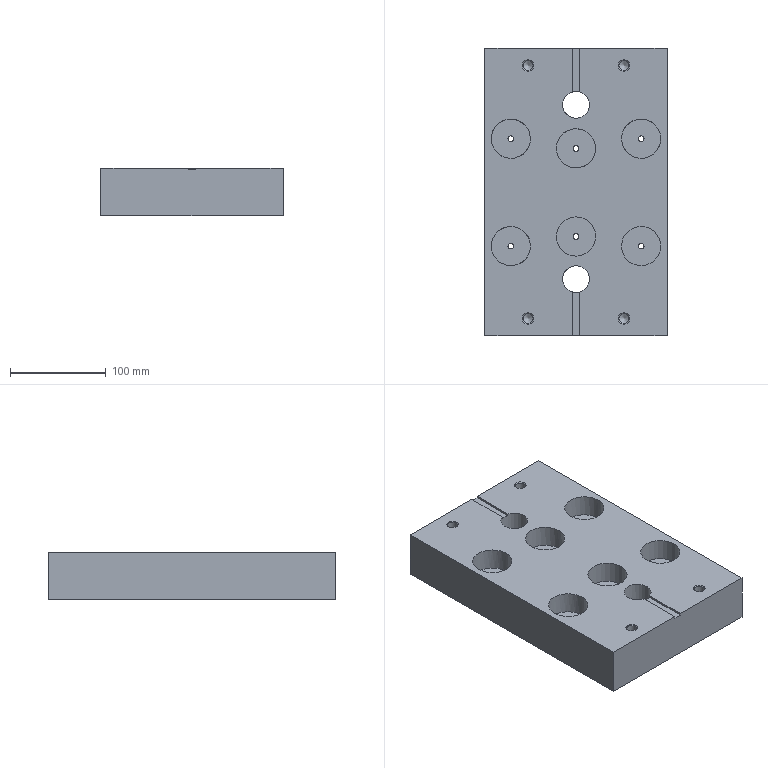Part | STEP file | gslz 2016.10.28-6_id1038_x_t | 1 solid | 44 faces | box 190 x 300 x 50 mm | volume 2589810 mm3 | plane 18 | cylinder 18 | cone 8 | commonest cylinder face diameters 6 x6 41 x6 10.3 x4 28 x2
STEP:
#1=CARTESIAN_POINT('',(4.,0.,-52.));
#2=VERTEX_POINT('',#1);
#3=CARTESIAN_POINT('',(-4.,0.,-52.));
#4=VERTEX_POINT('',#3);
#5=CARTESIAN_POINT('',(0.,0.,-52.));
#6=DIRECTION('',(-1.,0.,0.));
#7=VECTOR('',#6,1.);
#8=LINE('',#5,#7);
#9=EDGE_CURVE('',#2,#4,#8,.T.);
#10=ORIENTED_EDGE('',*,*,#9,.T.);
#11=CARTESIAN_POINT('',(-4.,0.,-50.));
#12=VERTEX_POINT('',#11);
#13=CARTESIAN_POINT('',(-4.,0.,-54.));
#14=DIRECTION('',(0.,0.,1.));
#15=VECTOR('',#14,1.);
#16=LINE('',#13,#15);
#17=EDGE_CURVE('',#4,#12,#16,.T.);
#18=ORIENTED_EDGE('',*,*,#17,.T.);
#19=CARTESIAN_POINT('',(-95.,0.,-50.));
#20=VERTEX_POINT('',#19);
#21=CARTESIAN_POINT('',(0.,0.,-50.));
#22=DIRECTION('',(1.,0.,0.));
#23=VECTOR('',#22,1.);
#24=LINE('',#21,#23);
#25=EDGE_CURVE('',#20,#12,#24,.T.);
#26=ORIENTED_EDGE('',*,*,#25,.F.);
#27=CARTESIAN_POINT('',(-95.,0.,-100.));
#28=VERTEX_POINT('',#27);
#29=CARTESIAN_POINT('',(-95.,0.,-221.492));
#30=DIRECTION('',(0.,0.,1.));
#31=VECTOR('',#30,1.);
#32=LINE('',#29,#31);
#33=EDGE_CURVE('',#28,#20,#32,.T.);
#34=ORIENTED_EDGE('',*,*,#33,.F.);
#35=CARTESIAN_POINT('',(95.,0.,-100.));
#36=VERTEX_POINT('',#35);
#37=CARTESIAN_POINT('',(0.,0.,-100.));
#38=DIRECTION('',(1.,0.,0.));
#39=VECTOR('',#38,1.);
#40=LINE('',#37,#39);
#41=EDGE_CURVE('',#28,#36,#40,.T.);
#42=ORIENTED_EDGE('',*,*,#41,.T.);
#43=CARTESIAN_POINT('',(95.,0.,-50.));
#44=VERTEX_POINT('',#43);
#45=CARTESIAN_POINT('',(95.,0.,-221.492));
#46=DIRECTION('',(0.,0.,1.));
#47=VECTOR('',#46,1.);
#48=LINE('',#45,#47);
#49=EDGE_CURVE('',#36,#44,#48,.T.);
#50=ORIENTED_EDGE('',*,*,#49,.T.);
#51=CARTESIAN_POINT('',(4.,0.,-50.));
#52=VERTEX_POINT('',#51);
#53=CARTESIAN_POINT('',(0.,0.,-50.));
#54=DIRECTION('',(1.,0.,0.));
#55=VECTOR('',#54,1.);
#56=LINE('',#53,#55);
#57=EDGE_CURVE('',#52,#44,#56,.T.);
#58=ORIENTED_EDGE('',*,*,#57,.F.);
#59=CARTESIAN_POINT('',(4.,0.,-54.));
#60=DIRECTION('',(0.,0.,1.));
#61=VECTOR('',#60,1.);
#62=LINE('',#59,#61);
#63=EDGE_CURVE('',#2,#52,#62,.T.);
#64=ORIENTED_EDGE('',*,*,#63,.F.);
#65=EDGE_LOOP('',(#10,#18,#26,#34,#42,#50,#58,#64));
#66=FACE_OUTER_BOUND('',#65,.T.);
#67=CARTESIAN_POINT('',(0.,0.,-221.492));
#68=DIRECTION('',(0.,-1.,0.));
#69=DIRECTION('',(0.,0.,1.));
#70=AXIS2_PLACEMENT_3D('',#67,#68,#69);
#71=PLANE('',#70);
#72=ADVANCED_FACE('',(#66),#71,.T.);
#73=CARTESIAN_POINT('',(-20.199,100.034,-50.));
#74=VERTEX_POINT('',#73);
#75=CARTESIAN_POINT('',(-0.000000001,103.534,-50.));
#76=DIRECTION('',(0.,0.,1.));
#77=DIRECTION('',(-1.,0.,0.));
#78=AXIS2_PLACEMENT_3D('',#75,#76,#77);
#79=CIRCLE('',#78,20.5);
#80=EDGE_CURVE('',#74,#74,#79,.T.);
#81=ORIENTED_EDGE('',*,*,#80,.F.);
#82=EDGE_LOOP('',(#81));
#83=FACE_BOUND('',#82,.T.);
#84=CARTESIAN_POINT('',(47.801,90.034,-50.));
#85=VERTEX_POINT('',#84);
#86=CARTESIAN_POINT('',(68.,93.534,-50.));
#87=DIRECTION('',(0.,0.,1.));
#88=DIRECTION('',(-1.,0.,0.));
#89=AXIS2_PLACEMENT_3D('',#86,#87,#88);
#90=CIRCLE('',#89,20.5);
#91=EDGE_CURVE('',#85,#85,#90,.T.);
#92=ORIENTED_EDGE('',*,*,#91,.F.);
#93=EDGE_LOOP('',(#92));
#94=FACE_BOUND('',#93,.T.);
#95=CARTESIAN_POINT('',(47.801,209.033,-50.));
#96=VERTEX_POINT('',#95);
#97=CARTESIAN_POINT('',(68.,205.533,-50.));
#98=DIRECTION('',(0.,0.,1.));
#99=DIRECTION('',(-1.,0.,0.));
#100=AXIS2_PLACEMENT_3D('',#97,#98,#99);
#101=CIRCLE('',#100,20.5);
#102=EDGE_CURVE('',#96,#96,#101,.T.);
#103=ORIENTED_EDGE('',*,*,#102,.F.);
#104=EDGE_LOOP('',(#103));
#105=FACE_BOUND('',#104,.T.);
#106=CARTESIAN_POINT('',(-20.199,199.033,-50.));
#107=VERTEX_POINT('',#106);
#108=CARTESIAN_POINT('',(0.,195.533,-50.));
#109=DIRECTION('',(0.,0.,-1.));
#110=DIRECTION('',(-1.,0.,0.));
#111=AXIS2_PLACEMENT_3D('',#108,#109,#110);
#112=CIRCLE('',#111,20.5);
#113=EDGE_CURVE('',#107,#107,#112,.T.);
#114=ORIENTED_EDGE('',*,*,#113,.T.);
#115=EDGE_LOOP('',(#114));
#116=FACE_BOUND('',#115,.T.);
#117=CARTESIAN_POINT('',(-47.801,90.034,-50.));
#118=VERTEX_POINT('',#117);
#119=CARTESIAN_POINT('',(-68.,93.534,-50.));
#120=DIRECTION('',(0.,0.,-1.));
#121=DIRECTION('',(-1.,0.,0.));
#122=AXIS2_PLACEMENT_3D('',#119,#120,#121);
#123=CIRCLE('',#122,20.5);
#124=EDGE_CURVE('',#118,#118,#123,.T.);
#125=ORIENTED_EDGE('',*,*,#124,.T.);
#126=EDGE_LOOP('',(#125));
#127=FACE_BOUND('',#126,.T.);
#128=CARTESIAN_POINT('',(4.,254.417,-50.));
#129=VERTEX_POINT('',#128);
#130=CARTESIAN_POINT('',(-4.,254.416,-50.));
#131=VERTEX_POINT('',#130);
#132=CARTESIAN_POINT('',(-0.000000005,241.,-50.));
#133=DIRECTION('',(0.,0.,-1.));
#134=DIRECTION('',(-1.,0.,0.));
#135=AXIS2_PLACEMENT_3D('',#132,#133,#134);
#136=CIRCLE('',#135,14.);
#137=EDGE_CURVE('',#129,#131,#136,.T.);
#138=ORIENTED_EDGE('',*,*,#137,.T.);
#139=CARTESIAN_POINT('',(-4.,300.,-50.));
#140=VERTEX_POINT('',#139);
#141=CARTESIAN_POINT('',(-4.,150.,-50.));
#142=DIRECTION('',(0.,-1.,0.));
#143=VECTOR('',#142,1.);
#144=LINE('',#141,#143);
#145=EDGE_CURVE('',#140,#131,#144,.T.);
#146=ORIENTED_EDGE('',*,*,#145,.F.);
#147=CARTESIAN_POINT('',(-95.,300.,-50.));
#148=VERTEX_POINT('',#147);
#149=CARTESIAN_POINT('',(0.,300.,-50.));
#150=DIRECTION('',(-1.,0.,0.));
#151=VECTOR('',#150,1.);
#152=LINE('',#149,#151);
#153=EDGE_CURVE('',#140,#148,#152,.T.);
#154=ORIENTED_EDGE('',*,*,#153,.T.);
#155=CARTESIAN_POINT('',(-95.,150.,-50.));
#156=DIRECTION('',(0.,1.,0.));
#157=VECTOR('',#156,1.);
#158=LINE('',#155,#157);
#159=EDGE_CURVE('',#20,#148,#158,.T.);
#160=ORIENTED_EDGE('',*,*,#159,.F.);
#161=ORIENTED_EDGE('',*,*,#25,.T.);
#162=CARTESIAN_POINT('',(-4.,45.584,-50.));
#163=VERTEX_POINT('',#162);
#164=CARTESIAN_POINT('',(-4.,150.,-50.));
#165=DIRECTION('',(0.,1.,0.));
#166=VECTOR('',#165,1.);
#167=LINE('',#164,#166);
#168=EDGE_CURVE('',#12,#163,#167,.T.);
#169=ORIENTED_EDGE('',*,*,#168,.T.);
#170=CARTESIAN_POINT('',(4.,45.583,-50.));
#171=VERTEX_POINT('',#170);
#172=CARTESIAN_POINT('',(0.000000001,59.,-50.));
#173=DIRECTION('',(0.,0.,-1.));
#174=DIRECTION('',(-1.,0.,0.));
#175=AXIS2_PLACEMENT_3D('',#172,#173,#174);
#176=CIRCLE('',#175,14.);
#177=EDGE_CURVE('',#163,#171,#176,.T.);
#178=ORIENTED_EDGE('',*,*,#177,.T.);
#179=CARTESIAN_POINT('',(4.,150.,-50.));
#180=DIRECTION('',(0.,1.,0.));
#181=VECTOR('',#180,1.);
#182=LINE('',#179,#181);
#183=EDGE_CURVE('',#52,#171,#182,.T.);
#184=ORIENTED_EDGE('',*,*,#183,.F.);
#185=ORIENTED_EDGE('',*,*,#57,.T.);
#186=CARTESIAN_POINT('',(95.,300.,-50.));
#187=VERTEX_POINT('',#186);
#188=CARTESIAN_POINT('',(95.,150.,-50.));
#189=DIRECTION('',(0.,1.,0.));
#190=VECTOR('',#189,1.);
#191=LINE('',#188,#190);
#192=EDGE_CURVE('',#44,#187,#191,.T.);
#193=ORIENTED_EDGE('',*,*,#192,.T.);
#194=CARTESIAN_POINT('',(4.,300.,-50.));
#195=VERTEX_POINT('',#194);
#196=CARTESIAN_POINT('',(0.,300.,-50.));
#197=DIRECTION('',(-1.,0.,0.));
#198=VECTOR('',#197,1.);
#199=LINE('',#196,#198);
#200=EDGE_CURVE('',#187,#195,#199,.T.);
#201=ORIENTED_EDGE('',*,*,#200,.T.);
#202=CARTESIAN_POINT('',(4.,150.,-50.));
#203=DIRECTION('',(0.,-1.,0.));
#204=VECTOR('',#203,1.);
#205=LINE('',#202,#204);
#206=EDGE_CURVE('',#195,#129,#205,.T.);
#207=ORIENTED_EDGE('',*,*,#206,.T.);
#208=EDGE_LOOP('',(#138,#146,#154,#160,#161,#169,#178,#184,#185,#193,#201,#207));
#209=FACE_BOUND('',#208,.T.);
#210=CARTESIAN_POINT('',(-47.801,202.033,-50.));
#211=VERTEX_POINT('',#210);
#212=CARTESIAN_POINT('',(-68.,205.533,-50.));
#213=DIRECTION('',(0.,0.,-1.));
#214=DIRECTION('',(-1.,0.,0.));
#215=AXIS2_PLACEMENT_3D('',#212,#213,#214);
#216=CIRCLE('',#215,20.5);
#217=EDGE_CURVE('',#211,#211,#216,.T.);
#218=ORIENTED_EDGE('',*,*,#217,.T.);
#219=EDGE_LOOP('',(#218));
#220=FACE_BOUND('',#219,.T.);
#221=CARTESIAN_POINT('',(44.,282.,-50.));
#222=VERTEX_POINT('',#221);
#223=CARTESIAN_POINT('',(50.,282.,-50.));
#224=DIRECTION('',(0.,0.,1.));
#225=DIRECTION('',(-1.,0.,0.));
#226=AXIS2_PLACEMENT_3D('',#223,#224,#225);
#227=CIRCLE('',#226,6.);
#228=EDGE_CURVE('',#222,#222,#227,.T.);
#229=ORIENTED_EDGE('',*,*,#228,.F.);
#230=EDGE_LOOP('',(#229));
#231=FACE_BOUND('',#230,.T.);
#232=CARTESIAN_POINT('',(-56.,282.,-50.));
#233=VERTEX_POINT('',#232);
#234=CARTESIAN_POINT('',(-50.,282.,-50.));
#235=DIRECTION('',(0.,0.,1.));
#236=DIRECTION('',(-1.,0.,0.));
#237=AXIS2_PLACEMENT_3D('',#234,#235,#236);
#238=CIRCLE('',#237,6.);
#239=EDGE_CURVE('',#233,#233,#238,.T.);
#240=ORIENTED_EDGE('',*,*,#239,.F.);
#241=EDGE_LOOP('',(#240));
#242=FACE_BOUND('',#241,.T.);
#243=CARTESIAN_POINT('',(44.,18.,-50.));
#244=VERTEX_POINT('',#243);
#245=CARTESIAN_POINT('',(50.,18.,-50.));
#246=DIRECTION('',(0.,0.,1.));
#247=DIRECTION('',(-1.,0.,0.));
#248=AXIS2_PLACEMENT_3D('',#245,#246,#247);
#249=CIRCLE('',#248,6.);
#250=EDGE_CURVE('',#244,#244,#249,.T.);
#251=ORIENTED_EDGE('',*,*,#250,.F.);
#252=EDGE_LOOP('',(#251));
#253=FACE_BOUND('',#252,.T.);
#254=CARTESIAN_POINT('',(-56.,18.,-50.));
#255=VERTEX_POINT('',#254);
#256=CARTESIAN_POINT('',(-50.,18.,-50.));
#257=DIRECTION('',(0.,0.,1.));
#258=DIRECTION('',(-1.,0.,0.));
#259=AXIS2_PLACEMENT_3D('',#256,#257,#258);
#260=CIRCLE('',#259,6.);
#261=EDGE_CURVE('',#255,#255,#260,.T.);
#262=ORIENTED_EDGE('',*,*,#261,.F.);
#263=EDGE_LOOP('',(#262));
#264=FACE_BOUND('',#263,.T.);
#265=CARTESIAN_POINT('',(-10.,150.,-50.));
#266=DIRECTION('',(0.,0.,-1.));
#267=DIRECTION('',(1.,0.,0.));
#268=AXIS2_PLACEMENT_3D('',#265,#266,#267);
#269=PLANE('',#268);
#270=ADVANCED_FACE('',(#83,#94,#105,#116,#127,#209,#220,#231,#242,#253,#264),#269,.F.);
#271=CARTESIAN_POINT('',(-4.,300.,-52.));
#272=VERTEX_POINT('',#271);
#273=CARTESIAN_POINT('',(4.,300.,-52.));
#274=VERTEX_POINT('',#273);
#275=CARTESIAN_POINT('',(0.,300.,-52.));
#276=DIRECTION('',(1.,0.,0.));
#277=VECTOR('',#276,1.);
#278=LINE('',#275,#277);
#279=EDGE_CURVE('',#272,#274,#278,.T.);
#280=ORIENTED_EDGE('',*,*,#279,.T.);
#281=CARTESIAN_POINT('',(4.,300.,-54.));
#282=DIRECTION('',(0.,0.,1.));
#283=VECTOR('',#282,1.);
#284=LINE('',#281,#283);
#285=EDGE_CURVE('',#274,#195,#284,.T.);
#286=ORIENTED_EDGE('',*,*,#285,.T.);
#287=ORIENTED_EDGE('',*,*,#200,.F.);
#288=CARTESIAN_POINT('',(95.,300.,-100.));
#289=VERTEX_POINT('',#288);
#290=CARTESIAN_POINT('',(95.,300.,-221.492));
#291=DIRECTION('',(0.,0.,1.));
#292=VECTOR('',#291,1.);
#293=LINE('',#290,#292);
#294=EDGE_CURVE('',#289,#187,#293,.T.);
#295=ORIENTED_EDGE('',*,*,#294,.F.);
#296=CARTESIAN_POINT('',(-95.,300.,-100.));
#297=VERTEX_POINT('',#296);
#298=CARTESIAN_POINT('',(0.,300.,-100.));
#299=DIRECTION('',(-1.,0.,0.));
#300=VECTOR('',#299,1.);
#301=LINE('',#298,#300);
#302=EDGE_CURVE('',#289,#297,#301,.T.);
#303=ORIENTED_EDGE('',*,*,#302,.T.);
#304=CARTESIAN_POINT('',(-95.,300.,-221.492));
#305=DIRECTION('',(0.,0.,1.));
#306=VECTOR('',#305,1.);
#307=LINE('',#304,#306);
#308=EDGE_CURVE('',#297,#148,#307,.T.);
#309=ORIENTED_EDGE('',*,*,#308,.T.);
#310=ORIENTED_EDGE('',*,*,#153,.F.);
#311=CARTESIAN_POINT('',(-4.,300.,-54.));
#312=DIRECTION('',(0.,0.,1.));
#313=VECTOR('',#312,1.);
#314=LINE('',#311,#313);
#315=EDGE_CURVE('',#272,#140,#314,.T.);
#316=ORIENTED_EDGE('',*,*,#315,.F.);
#317=EDGE_LOOP('',(#280,#286,#287,#295,#303,#309,#310,#316));
#318=FACE_OUTER_BOUND('',#317,.T.);
#319=CARTESIAN_POINT('',(0.,300.,-221.492));
#320=DIRECTION('',(0.,1.,0.));
#321=DIRECTION('',(0.,0.,-1.));
#322=AXIS2_PLACEMENT_3D('',#319,#320,#321);
#323=PLANE('',#322);
#324=ADVANCED_FACE('',(#318),#323,.T.);
#325=CARTESIAN_POINT('',(3.,103.534,-73.));
#326=VERTEX_POINT('',#325);
#327=CARTESIAN_POINT('',(-0.000000001,103.534,-73.));
#328=DIRECTION('',(0.,0.,1.));
#329=DIRECTION('',(1.,0.,0.));
#330=AXIS2_PLACEMENT_3D('',#327,#328,#329);
#331=CIRCLE('',#330,3.);
#332=EDGE_CURVE('',#326,#326,#331,.T.);
#333=ORIENTED_EDGE('',*,*,#332,.F.);
#334=EDGE_LOOP('',(#333));
#335=FACE_BOUND('',#334,.T.);
#336=CARTESIAN_POINT('',(-20.201,100.046,-73.));
#337=VERTEX_POINT('',#336);
#338=CARTESIAN_POINT('',(-20.199,100.034,-73.));
#339=VERTEX_POINT('',#338);
#340=CARTESIAN_POINT('',(-0.000000001,103.534,-73.));
#341=DIRECTION('',(0.,0.,-1.));
#342=DIRECTION('',(1.,0.,0.));
#343=AXIS2_PLACEMENT_3D('',#340,#341,#342);
#344=CIRCLE('',#343,20.5);
#345=EDGE_CURVE('',#337,#339,#344,.T.);
#346=ORIENTED_EDGE('',*,*,#345,.F.);
#347=CARTESIAN_POINT('',(-0.000000001,103.534,-73.));
#348=DIRECTION('',(0.,0.,-1.));
#349=DIRECTION('',(1.,0.,0.));
#350=AXIS2_PLACEMENT_3D('',#347,#348,#349);
#351=CIRCLE('',#350,20.5);
#352=EDGE_CURVE('',#339,#337,#351,.T.);
#353=ORIENTED_EDGE('',*,*,#352,.F.);
#354=EDGE_LOOP('',(#346,#353));
#355=FACE_BOUND('',#354,.T.);
#356=CARTESIAN_POINT('',(-0.000000001,103.534,-73.));
#357=DIRECTION('',(0.,0.,1.));
#358=DIRECTION('',(-1.,0.,0.));
#359=AXIS2_PLACEMENT_3D('',#356,#357,#358);
#360=PLANE('',#359);
#361=ADVANCED_FACE('',(#335,#355),#360,.T.);
#362=CARTESIAN_POINT('',(-65.,205.533,-73.));
#363=VERTEX_POINT('',#362);
#364=CARTESIAN_POINT('',(-68.,205.533,-73.));
#365=DIRECTION('',(0.,0.,1.));
#366=DIRECTION('',(1.,0.,0.));
#367=AXIS2_PLACEMENT_3D('',#364,#365,#366);
#368=CIRCLE('',#367,3.);
#369=EDGE_CURVE('',#363,#363,#368,.T.);
#370=ORIENTED_EDGE('',*,*,#369,.F.);
#371=EDGE_LOOP('',(#370));
#372=FACE_BOUND('',#371,.T.);
#373=CARTESIAN_POINT('',(-47.799,209.02,-73.));
#374=VERTEX_POINT('',#373);
#375=CARTESIAN_POINT('',(-47.801,202.033,-73.));
#376=VERTEX_POINT('',#375);
#377=CARTESIAN_POINT('',(-68.,205.533,-73.));
#378=DIRECTION('',(0.,0.,-1.));
#379=DIRECTION('',(1.,0.,0.));
#380=AXIS2_PLACEMENT_3D('',#377,#378,#379);
#381=CIRCLE('',#380,20.5);
#382=EDGE_CURVE('',#374,#376,#381,.T.);
#383=ORIENTED_EDGE('',*,*,#382,.F.);
#384=CARTESIAN_POINT('',(-68.,205.533,-73.));
#385=DIRECTION('',(0.,0.,-1.));
#386=DIRECTION('',(1.,0.,0.));
#387=AXIS2_PLACEMENT_3D('',#384,#385,#386);
#388=CIRCLE('',#387,20.5);
#389=EDGE_CURVE('',#376,#374,#388,.T.);
#390=ORIENTED_EDGE('',*,*,#389,.F.);
#391=EDGE_LOOP('',(#383,#390));
#392=FACE_BOUND('',#391,.T.);
#393=CARTESIAN_POINT('',(-107.5,104.533,-73.));
#394=DIRECTION('',(0.,0.,1.));
#395=DIRECTION('',(-1.,0.,0.));
#396=AXIS2_PLACEMENT_3D('',#393,#394,#395);
#397=PLANE('',#396);
#398=ADVANCED_FACE('',(#372,#392),#397,.T.);
#399=CARTESIAN_POINT('',(-65.,93.534,-73.));
#400=VERTEX_POINT('',#399);
#401=CARTESIAN_POINT('',(-68.,93.534,-73.));
#402=DIRECTION('',(0.,0.,1.));
#403=DIRECTION('',(1.,0.,0.));
#404=AXIS2_PLACEMENT_3D('',#401,#402,#403);
#405=CIRCLE('',#404,3.);
#406=EDGE_CURVE('',#400,#400,#405,.T.);
#407=ORIENTED_EDGE('',*,*,#406,.F.);
#408=EDGE_LOOP('',(#407));
#409=FACE_BOUND('',#408,.T.);
#410=CARTESIAN_POINT('',(-47.799,97.021,-73.));
#411=VERTEX_POINT('',#410);
#412=CARTESIAN_POINT('',(-47.801,90.034,-73.));
#413=VERTEX_POINT('',#412);
#414=CARTESIAN_POINT('',(-68.,93.534,-73.));
#415=DIRECTION('',(0.,0.,-1.));
#416=DIRECTION('',(1.,0.,0.));
#417=AXIS2_PLACEMENT_3D('',#414,#415,#416);
#418=CIRCLE('',#417,20.5);
#419=EDGE_CURVE('',#411,#413,#418,.T.);
#420=ORIENTED_EDGE('',*,*,#419,.F.);
#421=CARTESIAN_POINT('',(-68.,93.534,-73.));
#422=DIRECTION('',(0.,0.,-1.));
#423=DIRECTION('',(1.,0.,0.));
#424=AXIS2_PLACEMENT_3D('',#421,#422,#423);
#425=CIRCLE('',#424,20.5);
#426=EDGE_CURVE('',#413,#411,#425,.T.);
#427=ORIENTED_EDGE('',*,*,#426,.F.);
#428=EDGE_LOOP('',(#420,#427));
#429=FACE_BOUND('',#428,.T.);
#430=CARTESIAN_POINT('',(-107.5,96.534,-73.));
#431=DIRECTION('',(0.,0.,1.));
#432=DIRECTION('',(-1.,0.,0.));
#433=AXIS2_PLACEMENT_3D('',#430,#431,#432);
#434=PLANE('',#433);
#435=ADVANCED_FACE('',(#409,#429),#434,.T.);
#436=CARTESIAN_POINT('',(71.,93.534,-73.));
#437=VERTEX_POINT('',#436);
#438=CARTESIAN_POINT('',(68.,93.534,-73.));
#439=DIRECTION('',(0.,0.,1.));
#440=DIRECTION('',(1.,0.,0.));
#441=AXIS2_PLACEMENT_3D('',#438,#439,#440);
#442=CIRCLE('',#441,3.);
#443=EDGE_CURVE('',#437,#437,#442,.T.);
#444=ORIENTED_EDGE('',*,*,#443,.F.);
#445=EDGE_LOOP('',(#444));
#446=FACE_BOUND('',#445,.T.);
#447=CARTESIAN_POINT('',(47.799,90.046,-73.));
#448=VERTEX_POINT('',#447);
#449=CARTESIAN_POINT('',(47.801,90.034,-73.));
#450=VERTEX_POINT('',#449);
#451=CARTESIAN_POINT('',(68.,93.534,-73.));
#452=DIRECTION('',(0.,0.,-1.));
#453=DIRECTION('',(1.,0.,0.));
#454=AXIS2_PLACEMENT_3D('',#451,#452,#453);
#455=CIRCLE('',#454,20.5);
#456=EDGE_CURVE('',#448,#450,#455,.T.);
#457=ORIENTED_EDGE('',*,*,#456,.F.);
#458=CARTESIAN_POINT('',(68.,93.534,-73.));
#459=DIRECTION('',(0.,0.,-1.));
#460=DIRECTION('',(1.,0.,0.));
#461=AXIS2_PLACEMENT_3D('',#458,#459,#460);
#462=CIRCLE('',#461,20.5);
#463=EDGE_CURVE('',#450,#448,#462,.T.);
#464=ORIENTED_EDGE('',*,*,#463,.F.);
#465=EDGE_LOOP('',(#457,#464));
#466=FACE_BOUND('',#465,.T.);
#467=CARTESIAN_POINT('',(68.,93.534,-73.));
#468=DIRECTION('',(0.,0.,1.));
#469=DIRECTION('',(-1.,0.,0.));
#470=AXIS2_PLACEMENT_3D('',#467,#468,#469);
#471=PLANE('',#470);
#472=ADVANCED_FACE('',(#446,#466),#471,.T.);
#473=CARTESIAN_POINT('',(71.,205.533,-73.));
#474=VERTEX_POINT('',#473);
#475=CARTESIAN_POINT('',(68.,205.533,-73.));
#476=DIRECTION('',(0.,0.,1.));
#477=DIRECTION('',(1.,0.,0.));
#478=AXIS2_PLACEMENT_3D('',#475,#476,#477);
#479=CIRCLE('',#478,3.);
#480=EDGE_CURVE('',#474,#474,#479,.T.);
#481=ORIENTED_EDGE('',*,*,#480,.F.);
#482=EDGE_LOOP('',(#481));
#483=FACE_BOUND('',#482,.T.);
#484=CARTESIAN_POINT('',(47.799,202.046,-73.));
#485=VERTEX_POINT('',#484);
#486=CARTESIAN_POINT('',(47.801,209.033,-73.));
#487=VERTEX_POINT('',#486);
#488=CARTESIAN_POINT('',(68.,205.533,-73.));
#489=DIRECTION('',(0.,0.,-1.));
#490=DIRECTION('',(1.,0.,0.));
#491=AXIS2_PLACEMENT_3D('',#488,#489,#490);
#492=CIRCLE('',#491,20.5);
#493=EDGE_CURVE('',#485,#487,#492,.T.);
#494=ORIENTED_EDGE('',*,*,#493,.F.);
#495=CARTESIAN_POINT('',(68.,205.533,-73.));
#496=DIRECTION('',(0.,0.,-1.));
#497=DIRECTION('',(1.,0.,0.));
#498=AXIS2_PLACEMENT_3D('',#495,#496,#497);
#499=CIRCLE('',#498,20.5);
#500=EDGE_CURVE('',#487,#485,#499,.T.);
#501=ORIENTED_EDGE('',*,*,#500,.F.);
#502=EDGE_LOOP('',(#494,#501));
#503=FACE_BOUND('',#502,.T.);
#504=CARTESIAN_POINT('',(68.,205.533,-73.));
#505=DIRECTION('',(0.,0.,1.));
#506=DIRECTION('',(-1.,0.,0.));
#507=AXIS2_PLACEMENT_3D('',#504,#505,#506);
#508=PLANE('',#507);
#509=ADVANCED_FACE('',(#483,#503),#508,.T.);
#510=CARTESIAN_POINT('',(-3.,195.533,-73.));
#511=VERTEX_POINT('',#510);
#512=CARTESIAN_POINT('',(0.,195.533,-73.));
#513=DIRECTION('',(0.,0.,-1.));
#514=DIRECTION('',(-1.,0.,0.));
#515=AXIS2_PLACEMENT_3D('',#512,#513,#514);
#516=CIRCLE('',#515,3.);
#517=EDGE_CURVE('',#511,#511,#516,.T.);
#518=ORIENTED_EDGE('',*,*,#517,.T.);
#519=EDGE_LOOP('',(#518));
#520=FACE_BOUND('',#519,.T.);
#521=CARTESIAN_POINT('',(-20.199,199.033,-73.));
#522=VERTEX_POINT('',#521);
#523=CARTESIAN_POINT('',(-20.201,192.046,-73.));
#524=VERTEX_POINT('',#523);
#525=CARTESIAN_POINT('',(0.,195.533,-73.));
#526=DIRECTION('',(0.,0.,1.));
#527=DIRECTION('',(-1.,0.,0.));
#528=AXIS2_PLACEMENT_3D('',#525,#526,#527);
#529=CIRCLE('',#528,20.5);
#530=EDGE_CURVE('',#522,#524,#529,.T.);
#531=ORIENTED_EDGE('',*,*,#530,.T.);
#532=CARTESIAN_POINT('',(0.,195.533,-73.));
#533=DIRECTION('',(0.,0.,1.));
#534=DIRECTION('',(-1.,0.,0.));
#535=AXIS2_PLACEMENT_3D('',#532,#533,#534);
#536=CIRCLE('',#535,20.5);
#537=EDGE_CURVE('',#524,#522,#536,.T.);
#538=ORIENTED_EDGE('',*,*,#537,.T.);
#539=EDGE_LOOP('',(#531,#538));
#540=FACE_BOUND('',#539,.T.);
#541=CARTESIAN_POINT('',(0.,195.533,-73.));
#542=DIRECTION('',(0.,0.,-1.));
#543=DIRECTION('',(1.,0.,0.));
#544=AXIS2_PLACEMENT_3D('',#541,#542,#543);
#545=PLANE('',#544);
#546=ADVANCED_FACE('',(#520,#540),#545,.F.);
#547=CARTESIAN_POINT('',(-71.,93.534,-100.));
#548=VERTEX_POINT('',#547);
#549=CARTESIAN_POINT('',(-68.,93.534,-100.));
#550=DIRECTION('',(0.,0.,-1.));
#551=DIRECTION('',(-1.,0.,0.));
#552=AXIS2_PLACEMENT_3D('',#549,#550,#551);
#553=CIRCLE('',#552,3.);
#554=EDGE_CURVE('',#548,#548,#553,.T.);
#555=ORIENTED_EDGE('',*,*,#554,.F.);
#556=EDGE_LOOP('',(#555));
#557=FACE_BOUND('',#556,.T.);
#558=CARTESIAN_POINT('',(-71.,205.533,-100.));
#559=VERTEX_POINT('',#558);
#560=CARTESIAN_POINT('',(-68.,205.533,-100.));
#561=DIRECTION('',(0.,0.,-1.));
#562=DIRECTION('',(-1.,0.,0.));
#563=AXIS2_PLACEMENT_3D('',#560,#561,#562);
#564=CIRCLE('',#563,3.);
#565=EDGE_CURVE('',#559,#559,#564,.T.);
#566=ORIENTED_EDGE('',*,*,#565,.F.);
#567=EDGE_LOOP('',(#566));
#568=FACE_BOUND('',#567,.T.);
#569=CARTESIAN_POINT('',(65.,205.533,-100.));
#570=VERTEX_POINT('',#569);
#571=CARTESIAN_POINT('',(68.,205.533,-100.));
#572=DIRECTION('',(0.,0.,-1.));
#573=DIRECTION('',(-1.,0.,0.));
#574=AXIS2_PLACEMENT_3D('',#571,#572,#573);
#575=CIRCLE('',#574,3.);
#576=EDGE_CURVE('',#570,#570,#575,.T.);
#577=ORIENTED_EDGE('',*,*,#576,.F.);
#578=EDGE_LOOP('',(#577));
#579=FACE_BOUND('',#578,.T.);
#580=CARTESIAN_POINT('',(-3.,195.533,-100.));
#581=VERTEX_POINT('',#580);
#582=CARTESIAN_POINT('',(0.,195.533,-100.));
#583=DIRECTION('',(0.,0.,-1.));
#584=DIRECTION('',(-1.,0.,0.));
#585=AXIS2_PLACEMENT_3D('',#582,#583,#584);
#586=CIRCLE('',#585,3.);
#587=EDGE_CURVE('',#581,#581,#586,.T.);
#588=ORIENTED_EDGE('',*,*,#587,.F.);
#589=EDGE_LOOP('',(#588));
#590=FACE_BOUND('',#589,.T.);
#591=CARTESIAN_POINT('',(-3.,103.534,-100.));
#592=VERTEX_POINT('',#591);
#593=CARTESIAN_POINT('',(-0.000000001,103.534,-100.));
#594=DIRECTION('',(0.,0.,-1.));
#595=DIRECTION('',(-1.,0.,0.));
#596=AXIS2_PLACEMENT_3D('',#593,#594,#595);
#597=CIRCLE('',#596,3.);
#598=EDGE_CURVE('',#592,#592,#597,.T.);
#599=ORIENTED_EDGE('',*,*,#598,.F.);
#600=EDGE_LOOP('',(#599));
#601=FACE_BOUND('',#600,.T.);
#602=CARTESIAN_POINT('',(65.,93.534,-100.));
#603=VERTEX_POINT('',#602);
#604=CARTESIAN_POINT('',(68.,93.534,-100.));
#605=DIRECTION('',(0.,0.,-1.));
#606=DIRECTION('',(-1.,0.,0.));
#607=AXIS2_PLACEMENT_3D('',#604,#605,#606);
#608=CIRCLE('',#607,3.);
#609=EDGE_CURVE('',#603,#603,#608,.T.);
#610=ORIENTED_EDGE('',*,*,#609,.F.);
#611=EDGE_LOOP('',(#610));
#612=FACE_BOUND('',#611,.T.);
#613=CARTESIAN_POINT('',(-14.,241.,-100.));
#614=VERTEX_POINT('',#613);
#615=CARTESIAN_POINT('',(-0.000000005,241.,-100.));
#616=DIRECTION('',(0.,0.,-1.));
#617=DIRECTION('',(-1.,0.,0.));
#618=AXIS2_PLACEMENT_3D('',#615,#616,#617);
#619=CIRCLE('',#618,14.);
#620=EDGE_CURVE('',#614,#614,#619,.T.);
#621=ORIENTED_EDGE('',*,*,#620,.F.);
#622=EDGE_LOOP('',(#621));
#623=FACE_BOUND('',#622,.T.);
#624=CARTESIAN_POINT('',(-14.,59.,-100.));
#625=VERTEX_POINT('',#624);
#626=CARTESIAN_POINT('',(0.000000001,59.,-100.));
#627=DIRECTION('',(0.,0.,-1.));
#628=DIRECTION('',(-1.,0.,0.));
#629=AXIS2_PLACEMENT_3D('',#626,#627,#628);
#630=CIRCLE('',#629,14.);
#631=EDGE_CURVE('',#625,#625,#630,.T.);
#632=ORIENTED_EDGE('',*,*,#631,.F.);
#633=EDGE_LOOP('',(#632));
#634=FACE_BOUND('',#633,.T.);
#635=CARTESIAN_POINT('',(-95.,150.,-100.));
#636=DIRECTION('',(0.,1.,0.));
#637=VECTOR('',#636,1.);
#638=LINE('',#635,#637);
#639=EDGE_CURVE('',#28,#297,#638,.T.);
#640=ORIENTED_EDGE('',*,*,#639,.T.);
#641=ORIENTED_EDGE('',*,*,#302,.F.);
#642=CARTESIAN_POINT('',(95.,150.,-100.));
#643=DIRECTION('',(0.,1.,0.));
#644=VECTOR('',#643,1.);
#645=LINE('',#642,#644);
#646=EDGE_CURVE('',#36,#289,#645,.T.);
#647=ORIENTED_EDGE('',*,*,#646,.F.);
#648=ORIENTED_EDGE('',*,*,#41,.F.);
#649=EDGE_LOOP('',(#640,#641,#647,#648));
#650=FACE_BOUND('',#649,.T.);
#651=CARTESIAN_POINT('',(-140.,150.,-100.));
#652=DIRECTION('',(0.,0.,-1.));
#653=DIRECTION('',(1.,0.,0.));
#654=AXIS2_PLACEMENT_3D('',#651,#652,#653);
#655=PLANE('',#654);
#656=ADVANCED_FACE('',(#557,#568,#579,#590,#601,#612,#623,#634,#650),#655,.T.);
#657=ORIENTED_EDGE('',*,*,#426,.T.);
#658=ORIENTED_EDGE('',*,*,#419,.T.);
#659=EDGE_LOOP('',(#657,#658));
#660=FACE_BOUND('',#659,.T.);
#661=ORIENTED_EDGE('',*,*,#124,.F.);
#662=EDGE_LOOP('',(#661));
#663=FACE_BOUND('',#662,.T.);
#664=CARTESIAN_POINT('',(-68.,93.534,278.));
#665=DIRECTION('',(0.,0.,1.));
#666=DIRECTION('',(1.,0.,0.));
#667=AXIS2_PLACEMENT_3D('',#664,#665,#666);
#668=CYLINDRICAL_SURFACE('',#667,20.5);
#669=ADVANCED_FACE('',(#660,#663),#668,.F.);
#670=ORIENTED_EDGE('',*,*,#389,.T.);
#671=ORIENTED_EDGE('',*,*,#382,.T.);
#672=EDGE_LOOP('',(#670,#671));
#673=FACE_BOUND('',#672,.T.);
#674=ORIENTED_EDGE('',*,*,#217,.F.);
#675=EDGE_LOOP('',(#674));
#676=FACE_BOUND('',#675,.T.);
#677=CARTESIAN_POINT('',(-68.,205.533,-27.));
#678=DIRECTION('',(0.,0.,1.));
#679=DIRECTION('',(-1.,0.,0.));
#680=AXIS2_PLACEMENT_3D('',#677,#678,#679);
#681=CYLINDRICAL_SURFACE('',#680,20.5);
#682=ADVANCED_FACE('',(#673,#676),#681,.F.);
#683=ORIENTED_EDGE('',*,*,#352,.T.);
#684=ORIENTED_EDGE('',*,*,#345,.T.);
#685=EDGE_LOOP('',(#683,#684));
#686=FACE_BOUND('',#685,.T.);
#687=ORIENTED_EDGE('',*,*,#80,.T.);
#688=EDGE_LOOP('',(#687));
#689=FACE_BOUND('',#688,.T.);
#690=CARTESIAN_POINT('',(-0.000000001,103.534,-73.));
#691=DIRECTION('',(0.,0.,1.));
#692=DIRECTION('',(-1.,0.,0.));
#693=AXIS2_PLACEMENT_3D('',#690,#691,#692);
#694=CYLINDRICAL_SURFACE('',#693,20.5);
#695=ADVANCED_FACE('',(#686,#689),#694,.F.);
#696=ORIENTED_EDGE('',*,*,#537,.F.);
#697=ORIENTED_EDGE('',*,*,#530,.F.);
#698=EDGE_LOOP('',(#696,#697));
#699=FACE_BOUND('',#698,.T.);
#700=ORIENTED_EDGE('',*,*,#113,.F.);
#701=EDGE_LOOP('',(#700));
#702=FACE_BOUND('',#701,.T.);
#703=CARTESIAN_POINT('',(0.,195.533,-73.));
#704=DIRECTION('',(0.,0.,1.));
#705=DIRECTION('',(-1.,0.,0.));
#706=AXIS2_PLACEMENT_3D('',#703,#704,#705);
#707=CYLINDRICAL_SURFACE('',#706,20.5);
#708=ADVANCED_FACE('',(#699,#702),#707,.F.);
#709=ORIENTED_EDGE('',*,*,#500,.T.);
#710=ORIENTED_EDGE('',*,*,#493,.T.);
#711=EDGE_LOOP('',(#709,#710));
#712=FACE_BOUND('',#711,.T.);
#713=ORIENTED_EDGE('',*,*,#102,.T.);
#714=EDGE_LOOP('',(#713));
#715=FACE_BOUND('',#714,.T.);
#716=CARTESIAN_POINT('',(68.,205.533,-73.));
#717=DIRECTION('',(0.,0.,1.));
#718=DIRECTION('',(-1.,0.,0.));
#719=AXIS2_PLACEMENT_3D('',#716,#717,#718);
#720=CYLINDRICAL_SURFACE('',#719,20.5);
#721=ADVANCED_FACE('',(#712,#715),#720,.F.);
#722=ORIENTED_EDGE('',*,*,#463,.T.);
#723=ORIENTED_EDGE('',*,*,#456,.T.);
#724=EDGE_LOOP('',(#722,#723));
#725=FACE_BOUND('',#724,.T.);
#726=ORIENTED_EDGE('',*,*,#91,.T.);
#727=EDGE_LOOP('',(#726));
#728=FACE_BOUND('',#727,.T.);
#729=CARTESIAN_POINT('',(68.,93.534,-73.));
#730=DIRECTION('',(0.,0.,1.));
#731=DIRECTION('',(-1.,0.,0.));
#732=AXIS2_PLACEMENT_3D('',#729,#730,#731);
#733=CYLINDRICAL_SURFACE('',#732,20.5);
#734=ADVANCED_FACE('',(#725,#728),#733,.F.);
#735=ORIENTED_EDGE('',*,*,#192,.F.);
#736=ORIENTED_EDGE('',*,*,#49,.F.);
#737=ORIENTED_EDGE('',*,*,#646,.T.);
#738=ORIENTED_EDGE('',*,*,#294,.T.);
#739=EDGE_LOOP('',(#735,#736,#737,#738));
#740=FACE_OUTER_BOUND('',#739,.T.);
#741=CARTESIAN_POINT('',(95.,150.,-221.492));
#742=DIRECTION('',(1.,0.,0.));
#743=DIRECTION('',(0.,0.,-1.));
#744=AXIS2_PLACEMENT_3D('',#741,#742,#743);
#745=PLANE('',#744);
#746=ADVANCED_FACE('',(#740),#745,.T.);
#747=ORIENTED_EDGE('',*,*,#159,.T.);
#748=ORIENTED_EDGE('',*,*,#308,.F.);
#749=ORIENTED_EDGE('',*,*,#639,.F.);
#750=ORIENTED_EDGE('',*,*,#33,.T.);
#751=EDGE_LOOP('',(#747,#748,#749,#750));
#752=FACE_OUTER_BOUND('',#751,.T.);
#753=CARTESIAN_POINT('',(-95.,150.,-221.492));
#754=DIRECTION('',(-1.,0.,0.));
#755=DIRECTION('',(0.,0.,1.));
#756=AXIS2_PLACEMENT_3D('',#753,#754,#755);
#757=PLANE('',#756);
#758=ADVANCED_FACE('',(#752),#757,.T.);
#759=ORIENTED_EDGE('',*,*,#620,.T.);
#760=EDGE_LOOP('',(#759));
#761=FACE_BOUND('',#760,.T.);
#762=CARTESIAN_POINT('',(4.,254.417,-52.));
#763=VERTEX_POINT('',#762);
#764=CARTESIAN_POINT('',(-4.,254.416,-52.));
#765=VERTEX_POINT('',#764);
#766=CARTESIAN_POINT('',(-0.000000005,241.,-52.));
#767=DIRECTION('',(0.,0.,1.));
#768=DIRECTION('',(-1.,0.,0.));
#769=AXIS2_PLACEMENT_3D('',#766,#767,#768);
#770=CIRCLE('',#769,14.);
#771=EDGE_CURVE('',#763,#765,#770,.T.);
#772=ORIENTED_EDGE('',*,*,#771,.T.);
#773=CARTESIAN_POINT('',(-4.,254.416,-52.));
#774=DIRECTION('',(0.,0.,-1.));
#775=VECTOR('',#774,1.);
#776=LINE('',#773,#775);
#777=EDGE_CURVE('',#131,#765,#776,.T.);
#778=ORIENTED_EDGE('',*,*,#777,.F.);
#779=ORIENTED_EDGE('',*,*,#137,.F.);
#780=CARTESIAN_POINT('',(4.,254.417,-52.));
#781=DIRECTION('',(0.,0.,-1.));
#782=VECTOR('',#781,1.);
#783=LINE('',#780,#782);
#784=EDGE_CURVE('',#129,#763,#783,.T.);
#785=ORIENTED_EDGE('',*,*,#784,.T.);
#786=EDGE_LOOP('',(#772,#778,#779,#785));
#787=FACE_BOUND('',#786,.T.);
#788=CARTESIAN_POINT('',(-0.000000005,241.,-530.));
#789=DIRECTION('',(0.,0.,1.));
#790=DIRECTION('',(1.,0.,0.));
#791=AXIS2_PLACEMENT_3D('',#788,#789,#790);
#792=CYLINDRICAL_SURFACE('',#791,14.);
#793=ADVANCED_FACE('',(#761,#787),#792,.F.);
#794=ORIENTED_EDGE('',*,*,#631,.T.);
#795=EDGE_LOOP('',(#794));
#796=FACE_BOUND('',#795,.T.);
#797=CARTESIAN_POINT('',(-4.,45.584,-52.));
#798=VERTEX_POINT('',#797);
#799=CARTESIAN_POINT('',(4.,45.583,-52.));
#800=VERTEX_POINT('',#799);
#801=CARTESIAN_POINT('',(0.000000001,59.,-52.));
#802=DIRECTION('',(0.,0.,1.));
#803=DIRECTION('',(-1.,0.,0.));
#804=AXIS2_PLACEMENT_3D('',#801,#802,#803);
#805=CIRCLE('',#804,14.);
#806=EDGE_CURVE('',#798,#800,#805,.T.);
#807=ORIENTED_EDGE('',*,*,#806,.T.);
#808=CARTESIAN_POINT('',(4.,45.583,-52.));
#809=DIRECTION('',(0.,0.,-1.));
#810=VECTOR('',#809,1.);
#811=LINE('',#808,#810);
#812=EDGE_CURVE('',#171,#800,#811,.T.);
#813=ORIENTED_EDGE('',*,*,#812,.F.);
#814=ORIENTED_EDGE('',*,*,#177,.F.);
#815=CARTESIAN_POINT('',(-4.,45.584,-52.));
#816=DIRECTION('',(0.,0.,-1.));
#817=VECTOR('',#816,1.);
#818=LINE('',#815,#817);
#819=EDGE_CURVE('',#163,#798,#818,.T.);
#820=ORIENTED_EDGE('',*,*,#819,.T.);
#821=EDGE_LOOP('',(#807,#813,#814,#820));
#822=FACE_BOUND('',#821,.T.);
#823=CARTESIAN_POINT('',(0.000000001,59.,-380.));
#824=DIRECTION('',(0.,0.,1.));
#825=DIRECTION('',(1.,0.,0.));
#826=AXIS2_PLACEMENT_3D('',#823,#824,#825);
#827=CYLINDRICAL_SURFACE('',#826,14.);
#828=ADVANCED_FACE('',(#796,#822),#827,.F.);
#829=CARTESIAN_POINT('',(44.85,282.,-80.));
#830=VERTEX_POINT('',#829);
#831=CARTESIAN_POINT('',(50.,282.,-80.));
#832=DIRECTION('',(0.,0.,1.));
#833=DIRECTION('',(-1.,0.,0.));
#834=AXIS2_PLACEMENT_3D('',#831,#832,#833);
#835=CIRCLE('',#834,5.15);
#836=EDGE_CURVE('',#830,#830,#835,.T.);
#837=ORIENTED_EDGE('',*,*,#836,.T.);
#838=EDGE_LOOP('',(#837));
#839=FACE_BOUND('',#838,.T.);
#840=CARTESIAN_POINT('',(50.,282.,-83.094));
#841=VERTEX_POINT('',#840);
#842=VERTEX_LOOP('',#841);
#843=FACE_BOUND('',#842,.T.);
#844=CARTESIAN_POINT('',(50.,282.,-80.));
#845=DIRECTION('',(0.,0.,1.));
#846=DIRECTION('',(1.,0.,0.));
#847=AXIS2_PLACEMENT_3D('',#844,#845,#846);
#848=CONICAL_SURFACE('',#847,5.15,59.);
#849=ADVANCED_FACE('',(#839,#843),#848,.F.);
#850=CARTESIAN_POINT('',(55.15,282.,-50.85));
#851=VERTEX_POINT('',#850);
#852=CARTESIAN_POINT('',(50.,282.,-50.85));
#853=DIRECTION('',(0.,0.,-1.));
#854=DIRECTION('',(1.,0.,0.));
#855=AXIS2_PLACEMENT_3D('',#852,#853,#854);
#856=CIRCLE('',#855,5.15);
#857=EDGE_CURVE('',#851,#851,#856,.T.);
#858=ORIENTED_EDGE('',*,*,#857,.F.);
#859=EDGE_LOOP('',(#858));
#860=FACE_BOUND('',#859,.T.);
#861=ORIENTED_EDGE('',*,*,#836,.F.);
#862=EDGE_LOOP('',(#861));
#863=FACE_BOUND('',#862,.T.);
#864=CARTESIAN_POINT('',(50.,282.,-50.));
#865=DIRECTION('',(0.,0.,-1.));
#866=DIRECTION('',(-1.,0.,0.));
#867=AXIS2_PLACEMENT_3D('',#864,#865,#866);
#868=CYLINDRICAL_SURFACE('',#867,5.15);
#869=ADVANCED_FACE('',(#860,#863),#868,.F.);
#870=ORIENTED_EDGE('',*,*,#857,.T.);
#871=EDGE_LOOP('',(#870));
#872=FACE_BOUND('',#871,.T.);
#873=ORIENTED_EDGE('',*,*,#228,.T.);
#874=EDGE_LOOP('',(#873));
#875=FACE_BOUND('',#874,.T.);
#876=CARTESIAN_POINT('',(50.,282.,-50.));
#877=DIRECTION('',(0.,0.,1.));
#878=DIRECTION('',(-1.,0.,0.));
#879=AXIS2_PLACEMENT_3D('',#876,#877,#878);
#880=CONICAL_SURFACE('',#879,6.,45.);
#881=ADVANCED_FACE('',(#872,#875),#880,.F.);
#882=CARTESIAN_POINT('',(-55.15,282.,-80.));
#883=VERTEX_POINT('',#882);
#884=CARTESIAN_POINT('',(-50.,282.,-80.));
#885=DIRECTION('',(0.,0.,1.));
#886=DIRECTION('',(-1.,0.,0.));
#887=AXIS2_PLACEMENT_3D('',#884,#885,#886);
#888=CIRCLE('',#887,5.15);
#889=EDGE_CURVE('',#883,#883,#888,.T.);
#890=ORIENTED_EDGE('',*,*,#889,.T.);
#891=EDGE_LOOP('',(#890));
#892=FACE_BOUND('',#891,.T.);
#893=CARTESIAN_POINT('',(-50.,282.,-83.094));
#894=VERTEX_POINT('',#893);
#895=VERTEX_LOOP('',#894);
#896=FACE_BOUND('',#895,.T.);
#897=CARTESIAN_POINT('',(-50.,282.,-80.));
#898=DIRECTION('',(0.,0.,1.));
#899=DIRECTION('',(1.,0.,0.));
#900=AXIS2_PLACEMENT_3D('',#897,#898,#899);
#901=CONICAL_SURFACE('',#900,5.15,59.);
#902=ADVANCED_FACE('',(#892,#896),#901,.F.);
#903=CARTESIAN_POINT('',(-44.85,282.,-50.85));
#904=VERTEX_POINT('',#903);
#905=CARTESIAN_POINT('',(-50.,282.,-50.85));
#906=DIRECTION('',(0.,0.,-1.));
#907=DIRECTION('',(1.,0.,0.));
#908=AXIS2_PLACEMENT_3D('',#905,#906,#907);
#909=CIRCLE('',#908,5.15);
#910=EDGE_CURVE('',#904,#904,#909,.T.);
#911=ORIENTED_EDGE('',*,*,#910,.F.);
#912=EDGE_LOOP('',(#911));
#913=FACE_BOUND('',#912,.T.);
#914=ORIENTED_EDGE('',*,*,#889,.F.);
#915=EDGE_LOOP('',(#914));
#916=FACE_BOUND('',#915,.T.);
#917=CARTESIAN_POINT('',(-50.,282.,-50.));
#918=DIRECTION('',(0.,0.,-1.));
#919=DIRECTION('',(-1.,0.,0.));
#920=AXIS2_PLACEMENT_3D('',#917,#918,#919);
#921=CYLINDRICAL_SURFACE('',#920,5.15);
#922=ADVANCED_FACE('',(#913,#916),#921,.F.);
#923=ORIENTED_EDGE('',*,*,#910,.T.);
#924=EDGE_LOOP('',(#923));
#925=FACE_BOUND('',#924,.T.);
#926=ORIENTED_EDGE('',*,*,#239,.T.);
#927=EDGE_LOOP('',(#926));
#928=FACE_BOUND('',#927,.T.);
#929=CARTESIAN_POINT('',(-50.,282.,-50.));
#930=DIRECTION('',(0.,0.,1.));
#931=DIRECTION('',(-1.,0.,0.));
#932=AXIS2_PLACEMENT_3D('',#929,#930,#931);
#933=CONICAL_SURFACE('',#932,6.,45.);
#934=ADVANCED_FACE('',(#925,#928),#933,.F.);
#935=CARTESIAN_POINT('',(44.85,18.,-80.));
#936=VERTEX_POINT('',#935);
#937=CARTESIAN_POINT('',(50.,18.,-80.));
#938=DIRECTION('',(0.,0.,1.));
#939=DIRECTION('',(-1.,0.,0.));
#940=AXIS2_PLACEMENT_3D('',#937,#938,#939);
#941=CIRCLE('',#940,5.15);
#942=EDGE_CURVE('',#936,#936,#941,.T.);
#943=ORIENTED_EDGE('',*,*,#942,.T.);
#944=EDGE_LOOP('',(#943));
#945=FACE_BOUND('',#944,.T.);
#946=CARTESIAN_POINT('',(50.,18.,-83.094));
#947=VERTEX_POINT('',#946);
#948=VERTEX_LOOP('',#947);
#949=FACE_BOUND('',#948,.T.);
#950=CARTESIAN_POINT('',(50.,18.,-80.));
#951=DIRECTION('',(0.,0.,1.));
#952=DIRECTION('',(1.,0.,0.));
#953=AXIS2_PLACEMENT_3D('',#950,#951,#952);
#954=CONICAL_SURFACE('',#953,5.15,59.);
#955=ADVANCED_FACE('',(#945,#949),#954,.F.);
#956=CARTESIAN_POINT('',(55.15,18.,-50.85));
#957=VERTEX_POINT('',#956);
#958=CARTESIAN_POINT('',(50.,18.,-50.85));
#959=DIRECTION('',(0.,0.,-1.));
#960=DIRECTION('',(1.,0.,0.));
#961=AXIS2_PLACEMENT_3D('',#958,#959,#960);
#962=CIRCLE('',#961,5.15);
#963=EDGE_CURVE('',#957,#957,#962,.T.);
#964=ORIENTED_EDGE('',*,*,#963,.F.);
#965=EDGE_LOOP('',(#964));
#966=FACE_BOUND('',#965,.T.);
#967=ORIENTED_EDGE('',*,*,#942,.F.);
#968=EDGE_LOOP('',(#967));
#969=FACE_BOUND('',#968,.T.);
#970=CARTESIAN_POINT('',(50.,18.,-50.));
#971=DIRECTION('',(0.,0.,-1.));
#972=DIRECTION('',(-1.,0.,0.));
#973=AXIS2_PLACEMENT_3D('',#970,#971,#972);
#974=CYLINDRICAL_SURFACE('',#973,5.15);
#975=ADVANCED_FACE('',(#966,#969),#974,.F.);
#976=ORIENTED_EDGE('',*,*,#963,.T.);
#977=EDGE_LOOP('',(#976));
#978=FACE_BOUND('',#977,.T.);
#979=ORIENTED_EDGE('',*,*,#250,.T.);
#980=EDGE_LOOP('',(#979));
#981=FACE_BOUND('',#980,.T.);
#982=CARTESIAN_POINT('',(50.,18.,-50.));
#983=DIRECTION('',(0.,0.,1.));
#984=DIRECTION('',(-1.,0.,0.));
#985=AXIS2_PLACEMENT_3D('',#982,#983,#984);
#986=CONICAL_SURFACE('',#985,6.,45.);
#987=ADVANCED_FACE('',(#978,#981),#986,.F.);
#988=CARTESIAN_POINT('',(-55.15,18.,-80.));
#989=VERTEX_POINT('',#988);
#990=CARTESIAN_POINT('',(-50.,18.,-80.));
#991=DIRECTION('',(0.,0.,1.));
#992=DIRECTION('',(-1.,0.,0.));
#993=AXIS2_PLACEMENT_3D('',#990,#991,#992);
#994=CIRCLE('',#993,5.15);
#995=EDGE_CURVE('',#989,#989,#994,.T.);
#996=ORIENTED_EDGE('',*,*,#995,.T.);
#997=EDGE_LOOP('',(#996));
#998=FACE_BOUND('',#997,.T.);
#999=CARTESIAN_POINT('',(-50.,18.,-83.094));
#1000=VERTEX_POINT('',#999);
#1001=VERTEX_LOOP('',#1000);
#1002=FACE_BOUND('',#1001,.T.);
#1003=CARTESIAN_POINT('',(-50.,18.,-80.));
#1004=DIRECTION('',(0.,0.,1.));
#1005=DIRECTION('',(1.,0.,0.));
#1006=AXIS2_PLACEMENT_3D('',#1003,#1004,#1005);
#1007=CONICAL_SURFACE('',#1006,5.15,59.);
#1008=ADVANCED_FACE('',(#998,#1002),#1007,.F.);
#1009=CARTESIAN_POINT('',(-44.85,18.,-50.85));
#1010=VERTEX_POINT('',#1009);
#1011=CARTESIAN_POINT('',(-50.,18.,-50.85));
#1012=DIRECTION('',(0.,0.,-1.));
#1013=DIRECTION('',(1.,0.,0.));
#1014=AXIS2_PLACEMENT_3D('',#1011,#1012,#1013);
#1015=CIRCLE('',#1014,5.15);
#1016=EDGE_CURVE('',#1010,#1010,#1015,.T.);
#1017=ORIENTED_EDGE('',*,*,#1016,.F.);
#1018=EDGE_LOOP('',(#1017));
#1019=FACE_BOUND('',#1018,.T.);
#1020=ORIENTED_EDGE('',*,*,#995,.F.);
#1021=EDGE_LOOP('',(#1020));
#1022=FACE_BOUND('',#1021,.T.);
#1023=CARTESIAN_POINT('',(-50.,18.,-50.));
#1024=DIRECTION('',(0.,0.,-1.));
#1025=DIRECTION('',(-1.,0.,0.));
#1026=AXIS2_PLACEMENT_3D('',#1023,#1024,#1025);
#1027=CYLINDRICAL_SURFACE('',#1026,5.15);
#1028=ADVANCED_FACE('',(#1019,#1022),#1027,.F.);
#1029=ORIENTED_EDGE('',*,*,#1016,.T.);
#1030=EDGE_LOOP('',(#1029));
#1031=FACE_BOUND('',#1030,.T.);
#1032=ORIENTED_EDGE('',*,*,#261,.T.);
#1033=EDGE_LOOP('',(#1032));
#1034=FACE_BOUND('',#1033,.T.);
#1035=CARTESIAN_POINT('',(-50.,18.,-50.));
#1036=DIRECTION('',(0.,0.,1.));
#1037=DIRECTION('',(-1.,0.,0.));
#1038=AXIS2_PLACEMENT_3D('',#1035,#1036,#1037);
#1039=CONICAL_SURFACE('',#1038,6.,45.);
#1040=ADVANCED_FACE('',(#1031,#1034),#1039,.F.);
#1041=ORIENTED_EDGE('',*,*,#145,.T.);
#1042=ORIENTED_EDGE('',*,*,#777,.T.);
#1043=CARTESIAN_POINT('',(-4.,234.327,-52.));
#1044=DIRECTION('',(0.,-1.,0.));
#1045=VECTOR('',#1044,1.);
#1046=LINE('',#1043,#1045);
#1047=EDGE_CURVE('',#272,#765,#1046,.T.);
#1048=ORIENTED_EDGE('',*,*,#1047,.F.);
#1049=ORIENTED_EDGE('',*,*,#315,.T.);
#1050=EDGE_LOOP('',(#1041,#1042,#1048,#1049));
#1051=FACE_OUTER_BOUND('',#1050,.T.);
#1052=CARTESIAN_POINT('',(-4.,234.327,-54.));
#1053=DIRECTION('',(1.,0.,0.));
#1054=DIRECTION('',(0.,0.,-1.));
#1055=AXIS2_PLACEMENT_3D('',#1052,#1053,#1054);
#1056=PLANE('',#1055);
#1057=ADVANCED_FACE('',(#1051),#1056,.T.);
#1058=ORIENTED_EDGE('',*,*,#285,.F.);
#1059=CARTESIAN_POINT('',(4.,234.327,-52.));
#1060=DIRECTION('',(0.,-1.,0.));
#1061=VECTOR('',#1060,1.);
#1062=LINE('',#1059,#1061);
#1063=EDGE_CURVE('',#274,#763,#1062,.T.);
#1064=ORIENTED_EDGE('',*,*,#1063,.T.);
#1065=ORIENTED_EDGE('',*,*,#784,.F.);
#1066=ORIENTED_EDGE('',*,*,#206,.F.);
#1067=EDGE_LOOP('',(#1058,#1064,#1065,#1066));
#1068=FACE_OUTER_BOUND('',#1067,.T.);
#1069=CARTESIAN_POINT('',(4.,234.327,-54.));
#1070=DIRECTION('',(1.,0.,0.));
#1071=DIRECTION('',(0.,0.,1.));
#1072=AXIS2_PLACEMENT_3D('',#1069,#1070,#1071);
#1073=PLANE('',#1072);
#1074=ADVANCED_FACE('',(#1068),#1073,.F.);
#1075=ORIENTED_EDGE('',*,*,#771,.F.);
#1076=ORIENTED_EDGE('',*,*,#1063,.F.);
#1077=ORIENTED_EDGE('',*,*,#279,.F.);
#1078=ORIENTED_EDGE('',*,*,#1047,.T.);
#1079=EDGE_LOOP('',(#1075,#1076,#1077,#1078));
#1080=FACE_OUTER_BOUND('',#1079,.T.);
#1081=CARTESIAN_POINT('',(-0.0003999,234.327,-52.));
#1082=DIRECTION('',(0.,0.,-1.));
#1083=DIRECTION('',(0.,-1.,0.));
#1084=AXIS2_PLACEMENT_3D('',#1081,#1082,#1083);
#1085=PLANE('',#1084);
#1086=ADVANCED_FACE('',(#1080),#1085,.F.);
#1087=ORIENTED_EDGE('',*,*,#183,.T.);
#1088=ORIENTED_EDGE('',*,*,#812,.T.);
#1089=CARTESIAN_POINT('',(4.,65.673,-52.));
#1090=DIRECTION('',(0.,1.,0.));
#1091=VECTOR('',#1090,1.);
#1092=LINE('',#1089,#1091);
#1093=EDGE_CURVE('',#2,#800,#1092,.T.);
#1094=ORIENTED_EDGE('',*,*,#1093,.F.);
#1095=ORIENTED_EDGE('',*,*,#63,.T.);
#1096=EDGE_LOOP('',(#1087,#1088,#1094,#1095));
#1097=FACE_OUTER_BOUND('',#1096,.T.);
#1098=CARTESIAN_POINT('',(4.,65.673,-54.));
#1099=DIRECTION('',(-1.,0.,0.));
#1100=DIRECTION('',(0.,-1.,0.));
#1101=AXIS2_PLACEMENT_3D('',#1098,#1099,#1100);
#1102=PLANE('',#1101);
#1103=ADVANCED_FACE('',(#1097),#1102,.T.);
#1104=ORIENTED_EDGE('',*,*,#17,.F.);
#1105=CARTESIAN_POINT('',(-4.,65.673,-52.));
#1106=DIRECTION('',(0.,1.,0.));
#1107=VECTOR('',#1106,1.);
#1108=LINE('',#1105,#1107);
#1109=EDGE_CURVE('',#4,#798,#1108,.T.);
#1110=ORIENTED_EDGE('',*,*,#1109,.T.);
#1111=ORIENTED_EDGE('',*,*,#819,.F.);
#1112=ORIENTED_EDGE('',*,*,#168,.F.);
#1113=EDGE_LOOP('',(#1104,#1110,#1111,#1112));
#1114=FACE_OUTER_BOUND('',#1113,.T.);
#1115=CARTESIAN_POINT('',(-4.,65.673,-54.));
#1116=DIRECTION('',(-1.,0.,0.));
#1117=DIRECTION('',(0.,1.,0.));
#1118=AXIS2_PLACEMENT_3D('',#1115,#1116,#1117);
#1119=PLANE('',#1118);
#1120=ADVANCED_FACE('',(#1114),#1119,.F.);
#1121=ORIENTED_EDGE('',*,*,#806,.F.);
#1122=ORIENTED_EDGE('',*,*,#1109,.F.);
#1123=ORIENTED_EDGE('',*,*,#9,.F.);
#1124=ORIENTED_EDGE('',*,*,#1093,.T.);
#1125=EDGE_LOOP('',(#1121,#1122,#1123,#1124));
#1126=FACE_OUTER_BOUND('',#1125,.T.);
#1127=CARTESIAN_POINT('',(-0.0003999,65.673,-52.));
#1128=DIRECTION('',(0.,0.,-1.));
#1129=DIRECTION('',(0.,1.,0.));
#1130=AXIS2_PLACEMENT_3D('',#1127,#1128,#1129);
#1131=PLANE('',#1130);
#1132=ADVANCED_FACE('',(#1126),#1131,.F.);
#1133=ORIENTED_EDGE('',*,*,#443,.T.);
#1134=EDGE_LOOP('',(#1133));
#1135=FACE_BOUND('',#1134,.T.);
#1136=ORIENTED_EDGE('',*,*,#609,.T.);
#1137=EDGE_LOOP('',(#1136));
#1138=FACE_BOUND('',#1137,.T.);
#1139=CARTESIAN_POINT('',(68.,93.534,-50.));
#1140=DIRECTION('',(0.,0.,-1.));
#1141=DIRECTION('',(-1.,0.,0.));
#1142=AXIS2_PLACEMENT_3D('',#1139,#1140,#1141);
#1143=CYLINDRICAL_SURFACE('',#1142,3.);
#1144=ADVANCED_FACE('',(#1135,#1138),#1143,.F.);
#1145=ORIENTED_EDGE('',*,*,#332,.T.);
#1146=EDGE_LOOP('',(#1145));
#1147=FACE_BOUND('',#1146,.T.);
#1148=ORIENTED_EDGE('',*,*,#598,.T.);
#1149=EDGE_LOOP('',(#1148));
#1150=FACE_BOUND('',#1149,.T.);
#1151=CARTESIAN_POINT('',(-0.000000001,103.534,-50.));
#1152=DIRECTION('',(0.,0.,-1.));
#1153=DIRECTION('',(-1.,0.,0.));
#1154=AXIS2_PLACEMENT_3D('',#1151,#1152,#1153);
#1155=CYLINDRICAL_SURFACE('',#1154,3.);
#1156=ADVANCED_FACE('',(#1147,#1150),#1155,.F.);
#1157=ORIENTED_EDGE('',*,*,#587,.T.);
#1158=EDGE_LOOP('',(#1157));
#1159=FACE_BOUND('',#1158,.T.);
#1160=ORIENTED_EDGE('',*,*,#517,.F.);
#1161=EDGE_LOOP('',(#1160));
#1162=FACE_BOUND('',#1161,.T.);
#1163=CARTESIAN_POINT('',(0.,195.533,-50.));
#1164=DIRECTION('',(0.,0.,-1.));
#1165=DIRECTION('',(-1.,0.,0.));
#1166=AXIS2_PLACEMENT_3D('',#1163,#1164,#1165);
#1167=CYLINDRICAL_SURFACE('',#1166,3.);
#1168=ADVANCED_FACE('',(#1159,#1162),#1167,.F.);
#1169=ORIENTED_EDGE('',*,*,#480,.T.);
#1170=EDGE_LOOP('',(#1169));
#1171=FACE_BOUND('',#1170,.T.);
#1172=ORIENTED_EDGE('',*,*,#576,.T.);
#1173=EDGE_LOOP('',(#1172));
#1174=FACE_BOUND('',#1173,.T.);
#1175=CARTESIAN_POINT('',(68.,205.533,-50.));
#1176=DIRECTION('',(0.,0.,-1.));
#1177=DIRECTION('',(-1.,0.,0.));
#1178=AXIS2_PLACEMENT_3D('',#1175,#1176,#1177);
#1179=CYLINDRICAL_SURFACE('',#1178,3.);
#1180=ADVANCED_FACE('',(#1171,#1174),#1179,.F.);
#1181=ORIENTED_EDGE('',*,*,#369,.T.);
#1182=EDGE_LOOP('',(#1181));
#1183=FACE_BOUND('',#1182,.T.);
#1184=ORIENTED_EDGE('',*,*,#565,.T.);
#1185=EDGE_LOOP('',(#1184));
#1186=FACE_BOUND('',#1185,.T.);
#1187=CARTESIAN_POINT('',(-68.,205.533,-50.));
#1188=DIRECTION('',(0.,0.,-1.));
#1189=DIRECTION('',(-1.,0.,0.));
#1190=AXIS2_PLACEMENT_3D('',#1187,#1188,#1189);
#1191=CYLINDRICAL_SURFACE('',#1190,3.);
#1192=ADVANCED_FACE('',(#1183,#1186),#1191,.F.);
#1193=ORIENTED_EDGE('',*,*,#406,.T.);
#1194=EDGE_LOOP('',(#1193));
#1195=FACE_BOUND('',#1194,.T.);
#1196=ORIENTED_EDGE('',*,*,#554,.T.);
#1197=EDGE_LOOP('',(#1196));
#1198=FACE_BOUND('',#1197,.T.);
#1199=CARTESIAN_POINT('',(-68.,93.534,-50.));
#1200=DIRECTION('',(0.,0.,-1.));
#1201=DIRECTION('',(-1.,0.,0.));
#1202=AXIS2_PLACEMENT_3D('',#1199,#1200,#1201);
#1203=CYLINDRICAL_SURFACE('',#1202,3.);
#1204=ADVANCED_FACE('',(#1195,#1198),#1203,.F.);
#1205=CLOSED_SHELL('',(#72,#270,#324,#361,#398,#435,#472,#509,#546,#656,#669,#682,#695,#708,#721,#734,#746,#758,#793,#828,#849,#869,#881,#902,#922,#934,#955,#975,#987,#1008,#1028,#1040,#1057,#1074,#1086,#1103,#1120,#1132,#1144,#1156,#1168,#1180,#1192,#1204));
#1206=MANIFOLD_SOLID_BREP('',#1205);
#1207=(LENGTH_UNIT()NAMED_UNIT(*)SI_UNIT(.MILLI.,.METRE.));
#1208=UNCERTAINTY_MEASURE_WITH_UNIT(LENGTH_MEASURE(0.00002),#1207,'','');
#1209=(NAMED_UNIT(*)PLANE_ANGLE_UNIT()SI_UNIT($,.RADIAN.));
#1210=PLANE_ANGLE_MEASURE_WITH_UNIT(PLANE_ANGLE_MEASURE(0.01745),#1209);
#1211=DIMENSIONAL_EXPONENTS(0.,0.,0.,0.,0.,0.,0.);
#1212=(CONVERSION_BASED_UNIT('DEGREE',#1210)NAMED_UNIT(#1211)PLANE_ANGLE_UNIT());
#1213=(NAMED_UNIT(*)SI_UNIT($,.STERADIAN.)SOLID_ANGLE_UNIT());
#1214=(GEOMETRIC_REPRESENTATION_CONTEXT(3)GLOBAL_UNCERTAINTY_ASSIGNED_CONTEXT((#1208))GLOBAL_UNIT_ASSIGNED_CONTEXT((#1207,#1212,#1213))REPRESENTATION_CONTEXT('',''));
#1215=ADVANCED_BREP_SHAPE_REPRESENTATION('',(#1206),#1214);